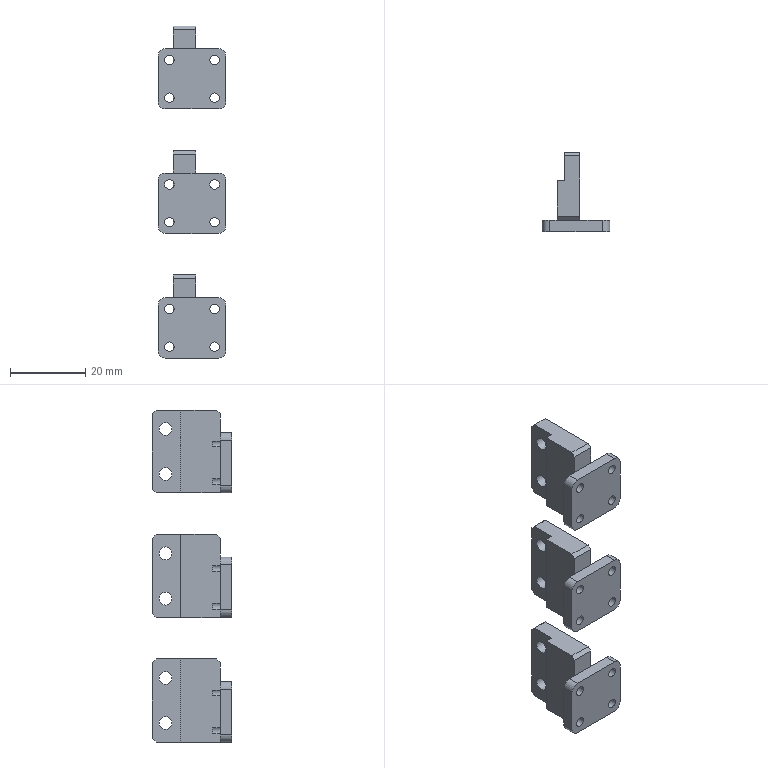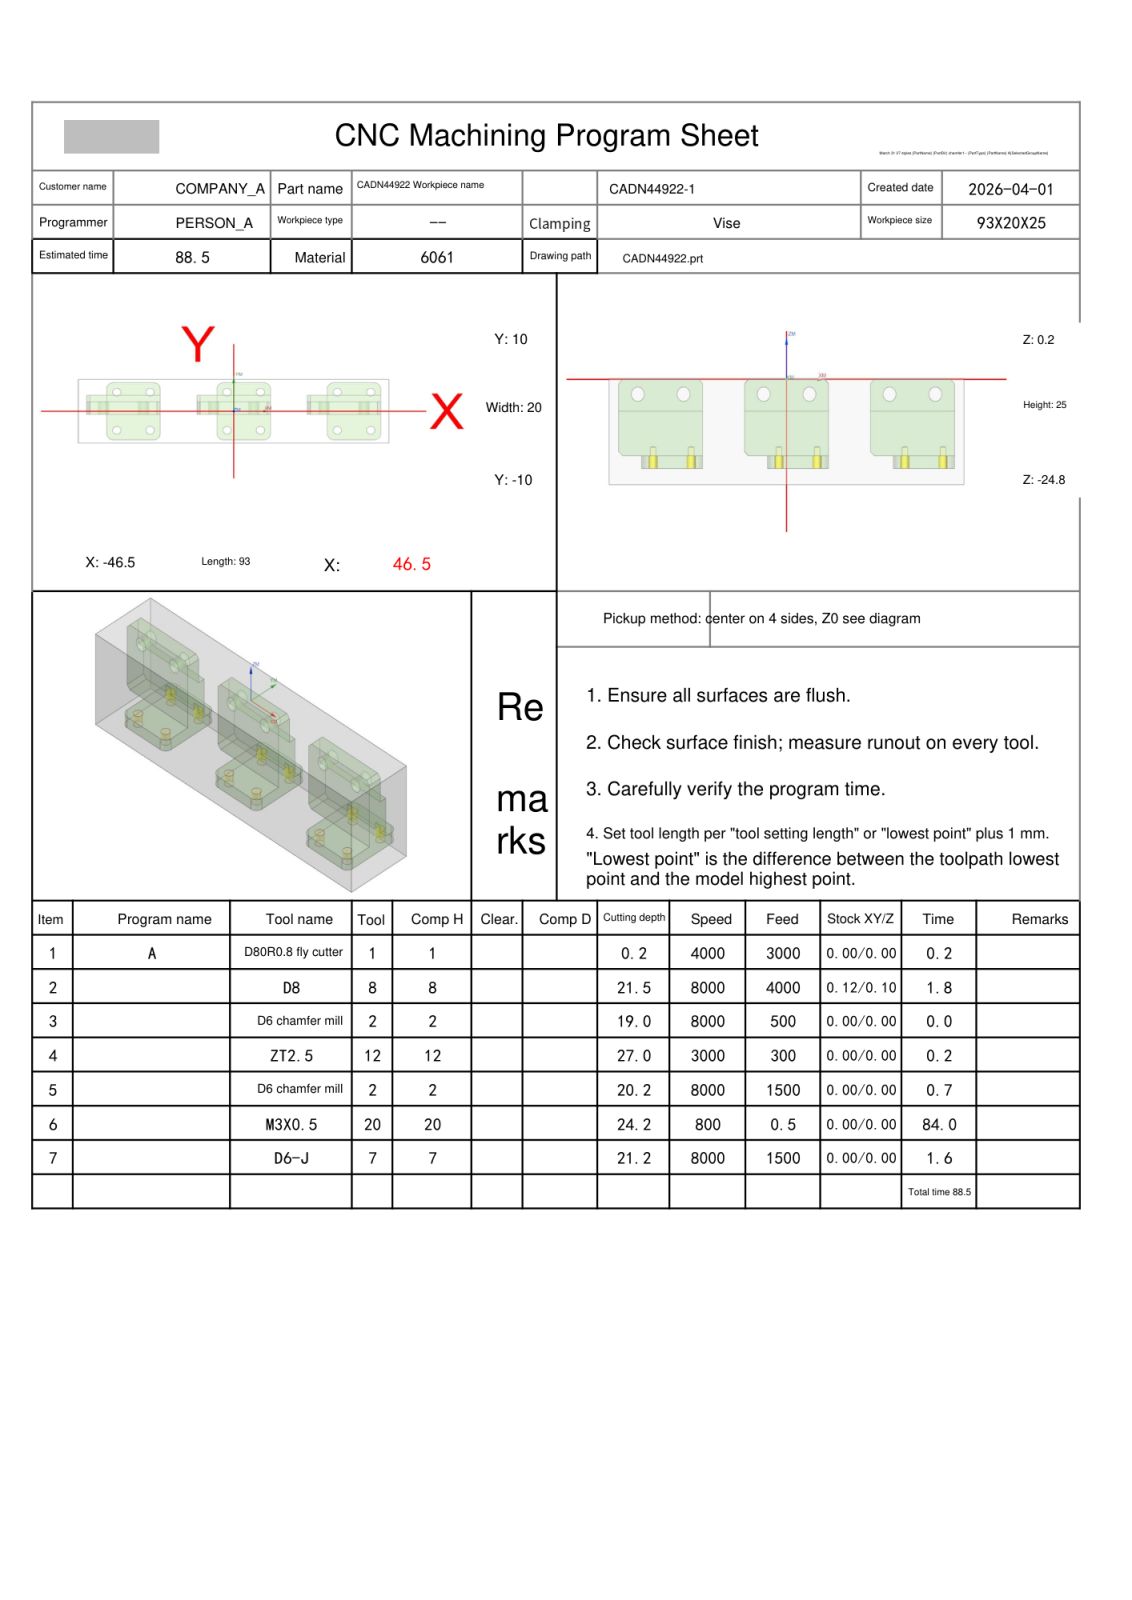NC program | NX | posted by the shop | part box 18 x 21 x 88 mm
Lines 42 to 965 of 4142:
N2 T08 M06
(D8  D=8. R=0. H=08 ce=0.12 di=0.10)
G00 G90 G54 X-55.984 Y.893 M03 S8000
G43 H08 Z20.
M08
Z-8.65
G01 X-55.886 Y.913 Z-9.275 F4000.
X-55.788 Y.933 Z-9.522
X-55.691 Y.953 Z-9.704
X-55.593 Y.973 Z-9.85
X-55.495 Y.993 Z-9.973
X-55.397 Y1.013 Z-10.078
X-55.299 Y1.033 Z-10.17
X-55.201 Y1.053 Z-10.25
X-55.103 Y1.073 Z-10.32
X-55.005 Y1.093 Z-10.382
X-54.907 Y1.114 Z-10.436
X-54.809 Y1.134 Z-10.483
X-54.711 Y1.154 Z-10.524
X-54.613 Y1.174 Z-10.558
X-54.515 Y1.194 Z-10.586
X-54.417 Y1.214 Z-10.61
X-54.319 Y1.234 Z-10.627
X-54.221 Y1.254 Z-10.64
X-54.123 Y1.274 Z-10.647
X-54.025 Y1.294 Z-10.65
G03 X-52.164 Y1.71 I-1.89 J12.828
X-51.742 Y2.726 I-1.554 J1.24
X-51.289 Y7.837 I-28.606 J5.111
X-51.291 Y8.113 I-29.059 J0.0
G01 Y8.202
G02 X-47.426 Y13.635 I5.75 J0.0
X-42.098 Y14.609 I5.697 J-16.103
X-32.642 Y14.767 I9.456 J-283.132
X-29.54 Y14.75 I0.0 J-283.29
G01 X44.939 Y14.729
G02 X50.005 Y11.176 I-.129 J-5.57
X51.093 Y5.793 I-14.693 J-5.771
X51.267 Y-3.345 I-239.376 J-9.138
X51.206 Y-8.763 I-239.55 J0.0
X47.747 Y-13.477 I-5.525 J.429
X42.45 Y-14.583 I-5.745 J14.271
X32.82 Y-14.772 I-9.629 J244.878
X29.493 Y-14.75 I0.0 J245.068
G01 X-44.987 Y-14.727
G02 X-50.03 Y-11.129 I.183 J5.591
X-51.097 Y-5.741 I15.012 J5.771
X-51.228 Y-2.403 I42.34 J3.339
X-51.135 Y.413 I42.471 J0.0
G03 X-50.486 Y7.409 I-193.07 J21.425
G02 X-46.65 Y12.332 I6.527 J-1.129
X-40.927 Y13.707 I6.529 J-14.588
X-32.915 Y13.956 I8.013 J-128.587
X-31.333 Y13.946 I0.0 J-128.836
G01 X43.227 Y13.93
G02 X48.701 Y10.316 I-.3 J-6.408
X50.166 Y4.775 I-13.357 J-6.497
X50.458 Y-3.345 I-112.899 J-8.12
X50.392 Y-7.216 I-113.19 J0.0
X46.802 Y-12.21 I-6.393 J.809
X41.187 Y-13.675 I-6.52 J13.493
X32.742 Y-13.964 I-8.445 J123.39
X30.714 Y-13.947 I0.0 J123.679
G01 X-43.285 Y-13.927
G02 X-48.694 Y-10.332 I.352 J6.396
X-50.172 Y-4.719 I13.363 J6.519
X-50.312 Y-1.795 I30.33 J2.925
X-50.173 Y1.111 I30.47 J0.0
X-49.729 Y6.084 I64.93 J-3.295
X-45.409 Y11.411 I7.394 J-1.582
X-39.138 Y12.893 I7.16 J-16.28
X-30.529 Y13.158 I8.609 J-140.056
X-28.744 Y13.146 I0.0 J-140.32
G01 X41.656 Y13.124
G02 X47.801 Y8.989 I-.403 J-7.234
X49.394 Y2.588 I-15.303 J-7.205
X49.628 Y-2.9 I-64.165 J-5.488
X49.569 Y-5.644 I-64.399 J0.0
X45.403 Y-11.344 I-7.201 J.891
X39.388 Y-12.861 I-7.037 J15.229
X30.46 Y-13.164 I-8.928 J131.417
X28.355 Y-13.147 I0.0 J131.72
G01 X-41.485 Y-13.133
G02 X-47.836 Y-8.926 I.241 J7.261
X-49.36 Y-2.003 I14.96 J6.923
X-49.358 Y-1.708 I16.484 J0.0
X-49.369 Y-.773 I38.904 J.935
X-48.975 Y4.753 I38.915 J0.0
X-44.084 Y10.609 I8.073 J-1.773
X-37.714 Y12.072 I7.44 J-17.796
X-28.909 Y12.355 I8.805 J-136.712
X-27.241 Y12.345 I0.0 J-136.995
G01 X40.039 Y12.323
G02 X46.809 Y8.02 I-.241 J-7.856
X48.159 Y5.123 I-3.267 J-3.285
X48.764 Y-2.392 I-46.345 J-7.515
X48.732 Y-4.123 I-46.951 J0.0
X44.329 Y-10.395 I-7.739 J.752
X38.016 Y-12.03 I-7.455 J15.78
X28.725 Y-12.364 I-9.291 J129.17
X26.585 Y-12.346 I0.0 J129.504
G01 X-39.975 Y-12.327
G02 X-47.003 Y-7.632 I.205 J7.916
X-48.407 Y-1.05 I14.735 J6.582
G01 X-48.406 Y-.95
G02 X-48.44 Y.203 I20.011 J1.154
X-48.12 Y3.769 I20.044 J0.0
X-48.135 Y4.318 I9.892 J.549
X-47.98 Y6.066 I9.907 J0.0
X-45.712 Y8.765 I4.256 J-1.274
X-37.316 Y11.193 I9.893 J-18.479
X-27.715 Y11.559 I9.602 J-125.917
X-25.806 Y11.544 I0.0 J-126.282
G01 X38.514 Y11.524
G02 X44.382 Y9.115 I-.093 J-8.581
G03 X45.066 Y8.98 I.887 J2.675
G02 X47.568 Y7.06 I-1.27 J-4.245
X48.12 Y4.998 I-4.216 J-2.233
X48.142 Y2.533 I-138.337 J-2.466
X48.074 Y-1.804 I-138.359 J0.0
X45.854 Y-7.572 I-8.758 J.06
X40.148 Y-10.643 I-7.988 J8.005
X32.366 Y-11.467 I-7.902 J37.493
X21.714 Y-11.551 I-10.652 J671.44
X19.887 Y-11.549 I0.0 J671.524
G01 X-38.513 Y-11.524
G02 X-46.253 Y-6.215 I.083 J8.418
X-47.08 Y-3.696 I21.506 J8.456
X-47.98 Y-2.066 I3.296 J2.883
G01 X-48.12 Y-1.
Y3.8
Y-1.
G03 X-46.913 Y-3.913 I4.433 J.13
X-44.908 Y-7.134 I34.469 J19.229
X-38.844 Y-10.524 I7.102 J5.587
X-32.41 Y-10.909 I6.434 J53.534
X-31.34 Y-10.898 I0.0 J53.919
G01 X29.14 Y-10.881
G03 X29.847 Y-10.885 I.706 J59.781
X38.153 Y-10.305 I0.0 J59.785
X43.773 Y-8.117 I-1.717 J12.722
X46.578 Y-4.211 I-4.972 J6.53
G01 X47.312 Y-3.451
X47.903 Y-2.319
X48.119 Y-1.062
X47.903 Y-2.319
X47.312 Y-3.451
G02 X44.255 Y-6.458 I-57.135 J55.023
X37.426 Y-9.418 I-8.966 J11.325
X28.955 Y-10.068 I-8.47 J54.924
X28.579 Y-10.066 I0.0 J55.573
G01 X18.099 Y-10.108
X-32.54 Y-10.08
G02 X-33.092 Y-10.085 I-.552 J31.482
X-38.749 Y-9.573 I0.0 J31.487
X-44.431 Y-5.798 I2.277 J9.59
G03 X-45.15 Y-4.945 I-6.698 J-4.918
G02 X-46.913 Y-3.913 I1.335 J4.305
G03 X-45.066 Y-4.98 I3.249 J3.495
G02 X-42.623 Y-6.82 I-24.322 J-34.837
G03 X-36.214 Y-9.123 I7.609 J11.103
X-28.807 Y-9.472 I7.407 J78.36
X-27.506 Y-9.461 I0.0 J78.709
G01 X27.214 Y-9.44
G03 X27.88 Y-9.443 I.666 J63.325
X36.467 Y-8.858 I0.0 J63.329
X44.555 Y-5.08 I-2.017 J14.86
G02 X45.262 Y-4.922 I.938 J-2.542
G01 X46.402 Y-4.347
X45.262 Y-4.922
G03 X42.996 Y-5.674 I.757 J-6.073
G02 X32.513 Y-8.399 I-11.731 J23.597
X22.846 Y-8.674 I-9.667 J169.882
X20.999 Y-8.664 I0.0 J170.156
G01 X-29.401 Y-8.642
G02 X-30.087 Y-8.648 I-.686 J42.
X-36.969 Y-8.08 I0.0 J42.005
X-42.722 Y-5.522 I3.391 J15.371
G03 X-43.802 Y-5.107 I-1.08 J-1.199
X-44.002 Y-5.12 I0.0 J-1.614
G01 X-45.066 Y-4.98
G03 X-43.144 Y-5.158 I3.33 J25.387
G02 X-39.892 Y-6.427 I-12.7 J-37.355
G03 X-32.05 Y-7.878 I8.484 J23.937
X-22.415 Y-8.041 I9.636 J284.651
X-19.573 Y-8.027 I0.0 J284.814
G01 X25.387 Y-7.999
G03 X26.124 Y-8.003 I.736 J68.243
X35.438 Y-7.365 I0.0 J68.247
X42.537 Y-5.145 I-5.252 J29.256
G01 X43.998 Y-5.12
X44.63 Y-5.021
G02 X42.923 Y-5.144 I-1.707 J11.757
X42.164 Y-5.12 I0.0 J11.881
G03 X38.031 Y-5.98 I4.598 J-32.461
G02 X27.071 Y-7.148 I-11.178 J52.874
X16.493 Y-7.23 I-10.578 J683.914
X14.352 Y-7.227 I0.0 J683.995
G01 X-27.168 Y-7.202
G02 X-27.827 Y-7.206 I-.659 J52.348
X-35.698 Y-6.611 I0.0 J52.353
X-40.837 Y-5.12 I6.892 J33.353
G01 X-43.397
G02 X-42.167 Y-5.095 I1.23 J-30.67
X-39.696 Y-5.195 I0.0 J-30.695
G03 X-33.218 Y-6.246 I15.885 J77.366
X-24.166 Y-6.591 I9.052 J118.887
X-22.747 Y-6.582 I0.0 J119.231
G01 X23.573 Y-6.561
G03 X24.392 Y-6.565 I.819 J79.441
X35.219 Y-5.824 I0.0 J79.446
G01 X38.762 Y-5.12
X42.202
G03 X39.693 Y-5.096 I-2.51 J-132.267
X35.211 Y-5.172 I0.0 J-132.291
G02 X20.435 Y-5.789 I-14.776 J176.515
X18.622 Y-5.78 I0.0 J177.132
G01 X-25.138 Y-5.762
G02 X-25.772 Y-5.765 I-.634 J70.43
X-35.285 Y-5.12 I0.0 J70.433
G01 X-40.485
X21.244 Y-5.126
X36.158 Y-5.12
X21.998
G02 X19.916 Y-4.721 I1.575 J13.876
G03 X14.411 Y-4.368 I-5.504 J-42.74
X13.376 Y-4.381 I0.0 J-43.093
G02 X10.998 Y-5.12 I-2.59 J4.136
G01 X-11.002
G02 X-13.232 Y-4.7 I2.272 J18.19
G03 X-18.518 Y-4.371 I-5.286 J-42.35
X-19.664 Y-4.386 I0.0 J-42.678
G01 X-20.755 Y-4.928
X-22.002 Y-5.12
X-20.755 Y-4.928
G02 X-18.492 Y-4.072 I3.398 J-5.57
X-16.287 Y-3.922 I2.206 J-16.071
X-13.635 Y-4.14 I0.0 J-16.222
G03 X-12.099 Y-4.966 I2.816 J3.395
G02 X-13.719 Y-4.062 I1.239 J4.125
G03 X-16.7 Y-3.375 I-2.981 J-6.124
X-17.019 Y-3.383 I0.0 J-6.811
G01 X-17.077
G03 X-18.794 Y-3.593 I0.0 J-7.099
G01 X-19.627 Y-4.368
G02 X-18.605 Y-3.451 I4.484 J-3.973
X-16.408 Y-3.018 I2.197 J-5.35
X-14.336 Y-3.401 I0.0 J-5.784
G03 X-13.659 Y-4.108 I3.262 J2.447
G02 X-14.354 Y-3.346 I1.716 J2.262
G03 X-16.7 Y-2.595 I-2.346 J-3.29
X-17.412 Y-2.658 I0.0 J-4.041
X-18.427 Y-2.991 I.135 J-2.126
G02 X-18.836 Y-3.605 I-3.058 J1.594
G03 X-18.402 Y-2.93 I-2.393 J2.014
G02 X-16.487 Y-2.316 I1.915 J-2.683
X-15.623 Y-2.431 I0.0 J-3.297
X-14.631 Y-2.909 I-.133 J-1.546
G03 X-14.276 Y-3.441 I2.812 J1.492
G02 X-14.775 Y-2.682 I7.022 J5.161
G03 X-16.661 Y-1.996 I-1.886 J-2.252
X-18.072 Y-2.357 I0.0 J-2.937
G01 X-18.457 Y-3.008
G02 X-17.93 Y-2.196 I2.254 J-.885
X-16.492 Y-1.778 I1.438 J-2.268
X-14.921 Y-2.286 I0.0 J-2.686
G01 X-14.664 Y-2.828
G03 X-16.378 Y-1.51 I-1.722 J-.466
X-16.7 Y-1.483 I-.322 J-1.937
X-18.001 Y-1.977 I0.0 J-1.963
G01 X-18.12 Y-2.387
G02 X-17.266 Y-1.422 I1.058 J-.076
X-16.516 Y-1.293 I.749 J-2.107
X-15.08 Y-1.815 I0.0 J-2.237
G01 X-14.857 Y-2.362
G03 X-15.183 Y-1.615 I-2.709 J-.739
X-16.582 Y-1.03 I-1.399 J-1.379
X-17.93 Y-1.566 I0.0 J-1.964
G01 X-18.075 Y-2.152
Y-2.14
G02 X-17.004 Y-.926 I1.223 J0.0
X-16.505 Y-.858 I.499 J-1.795
X-15.08 Y-1.521 I0.0 J-1.863
G01 X-14.995 Y-1.948
G03 X-16.063 Y-.706 I-1.264 J-.007
X-16.593 Y-.628 I-.529 J-1.759
X-17.827 Y-1.105 I0.0 J-1.837
X-17.995 Y-1.734 I2.468 J-.996
G02 X-17.747 Y-.951 I1.47 J-.035
X-16.513 Y-.463 I1.233 J-1.315
X-15.144 Y-1.094 I0.0 J-1.803
G01 X-15.039 Y-1.617
X-15.038 Y-1.573
G03 X-16.19 Y-.289 I-1.291 J0.0
X-16.629 Y-.226 I-.439 J-1.493
X-17.839 Y-.805 I0.0 J-1.556
G01 X-17.898 Y-1.231
X-17.903 Y-1.132
G02 X-17.167 Y-.201 I.957 J0.0
X-16.515 Y-.069 I.653 J-1.542
X-15.156 Y-.764 I0.0 J-1.674
G01 X-15.099 Y-1.159
X-15.097 Y-1.087
G03 X-15.991 Y.035 I-1.15 J0.0
X-16.576 Y.143 I-.585 J-1.532
X-17.826 Y-.436 I0.0 J-1.64
X-17.885 Y-.871 I1.594 J-.435
G01 X-17.883 Y-.94
X-17.899 Y-.768
G02 X-17.196 Y.159 I.962 J0.0
X-16.52 Y.303 I.676 J-1.505
X-15.151 Y-.426 I0.0 J-1.65
G01 X-15.12 Y-.868
X-15.108 Y-.702
G03 X-16.001 Y.407 I-1.136 J0.0
X-16.581 Y.518 I-.58 J-1.467
X-17.843 Y-.114 I0.0 J-1.577
X-17.883 Y-.657 I3.821 J-.553
G02 X-17.902 Y-.456 I1.04 J.201
X-17. Y.592 I1.06 J0.0
X-16.507 Y.669 I.493 J-1.545
X-15.151 Y-.063 I0.0 J-1.622
G01 X-15.12 Y-.505
X-15.107 Y-.336
G03 X-15.988 Y.772 I-1.138 J0.0
X-16.574 Y.884 I-.586 J-1.483
X-17.837 Y.261 I0.0 J-1.594
X-17.883 Y-.251 I2.83 J-.512
G01 Y-.307
G02 X-17.904 Y-.096 I1.046 J.212
X-17.007 Y.957 I1.067 J0.0
X-16.507 Y1.036 I.5 J-1.545
X-15.154 Y.309 I0.0 J-1.624
G01 X-15.12 Y-.139
X-15.107 Y.031
G03 X-15.978 Y1.136 I-1.137 J0.0
X-16.581 Y1.258 I-.603 J-1.431
X-17.849 Y.601 I0.0 J-1.553
G01 X-17.883 Y.155
X-17.897 Y.32
G02 X-17.188 Y1.264 I.983 J0.0
X-16.52 Y1.406 I.668 J-1.498
X-15.151 Y.67 I0.0 J-1.64
G01 X-15.12 Y.228
X-15.107 Y.398
G03 X-15.978 Y1.504 I-1.137 J0.0
X-16.573 Y1.618 I-.594 J-1.491
X-17.832 Y1.007 I0.0 J-1.605
X-17.885 Y.533 I2.129 J-.475
G01 X-17.882 Y.433
G02 X-17.903 Y.643 I1.045 J.211
X-17.031 Y1.692 I1.066 J0.0
X-16.516 Y1.775 I.515 J-1.554
X-15.154 Y1.046 I0.0 J-1.637
G01 X-15.12 Y.597
X-15.108 Y.763
G03 X-16.006 Y1.882 I-1.147 J0.0
X-16.574 Y1.987 I-.568 J-1.491
X-17.836 Y1.369 I0.0 J-1.596
X-17.882 Y.878 I2.964 J-.528
G01 X-17.899 Y1.059
G02 X-17.211 Y1.991 I.976 J0.0
X-16.509 Y2.154 I.702 J-1.427
X-15.14 Y1.373 I0.0 J-1.59
G01 X-15.12 Y.957
X-15.106 Y1.132
G03 X-15.98 Y2.242 I-1.142 J0.0
X-16.571 Y2.354 I-.591 J-1.496
X-17.833 Y1.745 I0.0 J-1.609
X-17.882 Y1.264 I2.318 J-.481
G01 Y1.251
X-17.899 Y1.432
G02 X-17.212 Y2.36 I.971 J0.0
X-16.524 Y2.509 I.689 J-1.517
X-15.162 Y1.803 I0.0 J-1.666
X-15.12 Y1.333 I-3.591 J-.559
G01 X-15.107 Y1.502
G03 X-15.98 Y2.611 I-1.141 J0.0
X-16.571 Y2.723 I-.59 J-1.494
X-17.833 Y2.11 I0.0 J-1.606
X-17.882 Y1.619 I2.454 J-.491
G01 Y1.617
X-17.894 Y1.777
G02 X-17.105 Y2.772 I1.022 J0.0
X-16.512 Y2.885 I.593 J-1.5
X-15.146 Y2.129 I0.0 J-1.613
G01 X-15.12 Y1.699
X-15.107 Y1.871
G03 X-15.979 Y2.979 I-1.14 J0.0
X-16.582 Y3.101 I-.603 J-1.425
X-17.848 Y2.443 I0.0 J-1.547
G01 X-17.882 Y1.997
X-17.896 Y2.162
G02 X-17.186 Y3.107 I.984 J0.0
X-16.52 Y3.248 I.666 J-1.499
X-15.151 Y2.511 I0.0 J-1.64
G01 X-15.12 Y2.07
X-15.107 Y2.24
G03 X-15.979 Y3.347 I-1.139 J0.0
X-16.571 Y3.459 I-.592 J-1.495
X-17.836 Y2.843 I0.0 J-1.608
X-17.882 Y2.324 I2.95 J-.519
G01 X-17.881 Y2.275
G02 X-17.902 Y2.484 I1.044 J.21
X-17.003 Y3.536 I1.065 J0.0
X-16.508 Y3.614 I.495 J-1.549
X-15.154 Y2.887 I0.0 J-1.626
G01 X-15.12 Y2.439
X-15.107 Y2.608
G03 X-15.979 Y3.715 I-1.139 J0.0
X-16.569 Y3.827 I-.59 J-1.49
X-17.835 Y3.207 I0.0 J-1.603
X-17.881 Y2.718 I3.153 J-.542
G01 X-17.894 Y2.878
G02 X-17.096 Y3.891 I1.042 J0.0
X-16.522 Y3.997 I.575 J-1.498
X-15.142 Y3.212 I0.0 J-1.604
G01 X-15.12 Y2.79
X-15.109 Y2.952
G03 X-16.129 Y4.155 I-1.219 J0.0
X-16.576 Y4.22 I-.447 J-1.49
X-17.845 Y3.564 I0.0 J-1.556
G01 X-17.881 Y3.111
X-17.891 Y3.257
G02 X-17.003 Y4.315 I1.075 J0.0
X-16.518 Y4.391 I.485 J-1.513
X-15.141 Y3.596 I0.0 J-1.589
G01 X-15.12 Y3.176
X-15.11 Y3.331
G03 X-16.267 Y4.586 I-1.259 J0.0
X-16.594 Y4.622 I-.327 J-1.462
X-17.852 Y3.937 I0.0 J-1.498
G01 X-17.881 Y3.422
G02 X-17.899 Y3.622 I1.109 J.2
X-16.936 Y4.737 I1.126 J0.0
X-16.517 Y4.793 I.419 J-1.531
X-15.143 Y4. I0.0 J-1.587
G01 X-15.12 Y3.497
G03 X-15.103 Y3.706 I-1.287 J.209
X-16.407 Y5.009 I-1.304 J0.0
G01 X-16.409
G03 X-16.634 Y5.027 I-.225 J-1.382
X-17.864 Y4.297 I0.0 J-1.4
G01 X-17.881 Y3.743
G02 X-17.905 Y3.987 I1.196 J.244
X-17.661 Y4.719 I1.221 J0.0
X-16.52 Y5.21 I1.142 J-1.082
X-15.137 Y4.386 I0.0 J-1.573
G01 X-15.12 Y3.912
G03 X-15.102 Y4.124 I-1.277 J.212
X-16.395 Y5.418 I-1.295 J0.0
X-16.627 Y5.437 I-.232 J-1.402
X-17.859 Y4.725 I0.0 J-1.421
G01 X-17.88 Y4.226
G02 X-17.789 Y5.659 I43.024 J-2.025
G03 X-20.287 Y9.349 I-4.719 J-.503
X-25.102 Y10.687 I-5.356 J-9.946
X-30.065 Y10.87 I-4.962 J-67.001
X-38.594 Y10.327 I0.0 J-67.184
X-43.183 Y9.12 I3.439 J-22.406
X-43.671 Y9.143 I-.488 J-5.23
X-46.06 Y8.568 I0.0 J-5.253
G02 X-43.671 Y9.143 I2.389 J-4.678
X-43.183 Y9.12 I0.0 J-5.252
G03 X-39.086 Y9.472 I-.17 J26.04
G02 X-30.028 Y10.034 I9.058 J-72.709
X-26.391 Y9.943 I0.0 J-73.271
X-22.46 Y9.12 I-.744 J-13.344
X-22.173 Y9.129 I.287 J-4.516
X-19.087 Y7.913 I0.0 J-4.525
X-17.876 Y4.866 I-3.229 J-3.047
G01 X-17.88 Y4.678
X-17.877 Y4.858
G03 X-19.087 Y7.913 I-4.462 J0.0
X-22.174 Y9.129 I-3.087 J-3.312
X-22.46 Y9.12 I0.0 J-4.527
G02 X-27.808 Y9.347 I5.551 J193.932
G03 X-29.304 Y9.359 I-1.496 J-90.788
X-35.89 Y9.12 I0.0 J-90.8
G01 X-42.37
X-23.25
G03 X-22.953 Y9.252 I-.008 J.419
G01 X-22.416 Y9.848
X-21.364 Y11.016 Z-10.55
X-20.921 Y11.509
X-20.87 Y11.556
X-20.813 Y11.593
X-20.75 Y11.62
X-16.09 Y13.174
X-15.623 Y13.325
X-15.153 Y13.467
X-14.681 Y13.6
X-14.206 Y13.725
X-13.934 Y13.789
X-13.66 Y13.844
X-13.385 Y13.889
X-13.108 Y13.925
X-12.83 Y13.951
X-12.551 Y13.968
X-12.271 Y13.975
X37.312 Y14.411
X37.689 Y14.409
X38.065 Y14.395
X38.441 Y14.371
X38.816 Y14.336
X39.189 Y14.29
X39.562 Y14.233
X39.932 Y14.165
X40.3 Y14.087
X40.666 Y13.998
X41.029 Y13.898
X41.389 Y13.787
X41.746 Y13.666
X42.099 Y13.535
X44.544 Y12.585
X44.602 Y12.557
X44.655 Y12.52
X44.701 Y12.475
X44.739 Y12.423
X44.768 Y12.365
X44.788 Y12.304
X44.798 Y12.24
X44.886 Y10.999
X44.996 Y9.431 Z-10.65
G02 X44.595 Y9.045 I-.4 J.015
G01 X44.544 Y9.048
G02 X42.149 Y9.958 I10.936 J32.404
G03 X36.185 Y10.837 I-5.965 J-19.782
G01 X36.076
G03 X26.709 Y10.908 I-9.367 J-615.807
G01 X26.157
X-10.64 Y10.888
G03 X-13.243 Y8.707 I.895 J-3.712
G02 X-13.913 Y7.913 I-1.332 J.445
G03 X-15.12 Y5.002 I3.22 J-3.04
G01 Y4.362
G02 X-15.134 Y4.738 I5.032 J.377
X-14.568 Y7.06 I5.046 J0.0
X-11.746 Y9.152 I4.124 J-2.613
X-5.91 Y10.013 I5.892 J-19.741
X.442 Y10.12 I6.352 J-188.533
X2.569 Y10.108 I0.0 J-188.64
G01 X34.488 Y10.084
G02 X34.898 Y10.087 I.409 J-23.458
X41.566 Y9.12 I0.0 J-23.462
X42.575 Y9.144 I1.008 J-20.805
X44.478 Y9.057 I0.0 J-20.829
G03 X42.575 Y9.144 I-1.903 J-20.742
X41.566 Y9.12 I0.0 J-20.829
G02 X36.368 Y9.358 I1.498 J89.466
G03 X25.671 Y9.474 I-10.697 J-492.923
X23.089 Y9.467 I0.0 J-493.039
G01 X-3.07 Y9.443
G03 X-8.415 Y9.12 I.403 J-51.051
G01 X-10.998
G03 X-13.06 Y8.568 I.172 J-4.77
G02 X-10.998 Y9.12 I2.233 J-4.216
G01 X11.002
G03 X17.523 Y8.683 I6.521 J48.497
X18.201 Y8.688 I0.0 J48.934
G01 X20.245 Y8.695
G02 X22.002 Y9.12 I1.87 J-3.883
G01 X40.562
G03 X40.962 Y9.52 I0.0 J.4
X40.776 Y9.858 I-.4 J0.0
G01 X40.183 Y10.233
X38.855 Y11.075 Z-10.55
X38.586 Y11.246
X38.537 Y11.272
X38.484 Y11.292
X38.43 Y11.304
X38.374 Y11.308
X21.793 Y11.374
X21.726 Y11.369
X21.662 Y11.353
X21.601 Y11.326
X21.545 Y11.29
X21.496 Y11.245
X21.455 Y11.192
X21.424 Y11.133
X21.385 Y11.044
X20.761 Y9.602 Z-10.65
X20.431 Y8.851
G02 X19.338 Y8.423 I-1.244 J1.567
X15.814 Y8.167 I-3.524 J24.144
X13.486 Y8.278 I0.0 J24.4
G03 X12.066 Y8.98 I-3.028 J-4.34
G02 X13.655 Y8.153 I-1.738 J-5.282
G03 X16.937 Y7.576 I3.282 J9.052
X17.91 Y7.626 I0.0 J9.629
G01 X18.026 Y7.623
G03 X19.002 Y7.828 I0.0 J2.426
G02 X20.088 Y8.629 I3.848 J-4.077
G03 X18.946 Y7.755 I1.868 J-3.621
G02 X16.47 Y7.195 I-2.476 J5.203
X15.758 Y7.239 I0.0 J5.762
X14.179 Y7.586 I.001 J3.771
G03 X13.406 Y8.303 I-2.221 J-1.622
G02 X14.24 Y7.498 I-1.443 J-2.332
G03 X16.675 Y6.761 I2.435 J3.653
X17.295 Y6.805 I0.0 J4.39
X18.495 Y7.142 I-.02 J2.375
G01 X19.079 Y7.903
G02 X18.244 Y6.919 I-3.856 J2.424
X16.461 Y6.468 I-1.783 J3.296
X14.664 Y6.927 I0.0 J3.748
G01 X14.178 Y7.568
G03 X14.907 Y6.656 I4.149 J2.569
X16.63 Y6.124 I1.722 J2.52
X18.186 Y6.55 I0.0 J3.053
G01 X18.481 Y7.123
G02 X18.056 Y6.384 I-2.15 J.742
X16.499 Y5.887 I-1.557 J2.189
X14.828 Y6.47 I0.0 J2.686
G01 X14.607 Y6.966
G03 X16.134 Y5.662 I1.682 J.423
X16.655 Y5.602 I.52 J2.218
X17.976 Y6.024 I0.0 J2.278
G01 X18.285 Y6.705
G02 X17.858 Y5.861 I-2.25 J.609
X16.487 Y5.407 I-1.371 J1.843
X15.077 Y5.89 I0.0 J2.297
G01 X14.796 Y6.51
G03 X15.24 Y5.643 I2.099 J.527
X16.581 Y5.145 I1.341 J1.558
X17.9 Y5.625 I0.0 J2.055
X18.02 Y6.066 I-1.34 J.602
G01 X18.021 Y6.045
G02 X17.37 Y5.156 I-.932 J0.0
X16.518 Y4.96 I-.851 J1.746
X15.07 Y5.607 I0.0 J1.943
G01 X14.98 Y6.066
X14.979 Y6.045
G03 X15.968 Y4.835 I1.235 J0.0
X16.591 Y4.724 I.623 J1.684
X17.873 Y5.263 I0.0 J1.795
X17.996 Y5.879 I-2.982 J.914
G01 X17.997 Y5.818
G02 X17.784 Y5.084 I-1.37 J0.0
X16.513 Y4.555 I-1.271 J1.263
X15.113 Y5.229 I0.0 J1.792
G01 X15.035 Y5.646
G03 X16.177 Y4.389 I1.271 J.008
X16.604 Y4.333 I.427 J1.614
X17.825 Y4.864 I0.0 J1.67
X17.943 Y5.478 I-5.741 J1.419
G01 X17.945 Y5.4
G02 X16.794 Y4.202 I-1.199 J0.0
X16.485 Y4.173 I-.309 J1.628
X15.164 Y4.83 I0.0 J1.657
G01 X15.078 Y5.316
X15.076 Y5.244
G03 X16.16 Y4.014 I1.239 J0.0
X16.593 Y3.954 I.432 J1.526
X17.832 Y4.55 I0.0 J1.586
X17.88 Y5.002 I-2.768 J.526
G01 X17.892 Y4.855
G02 X17.191 Y3.938 I-.95 J0.0
X16.514 Y3.791 I-.677 J1.494
X15.149 Y4.522 I0.0 J1.64
G01 X15.12 Y4.959
X15.107 Y4.791
G03 X15.991 Y3.69 I1.128 J0.0
X16.585 Y3.573 I.594 J1.446
X17.844 Y4.209 I0.0 J1.563
G01 X17.88 Y4.664
X17.894 Y4.501
G02 X17.165 Y3.557 I-.975 J0.0
X16.509 Y3.417 I-.655 J1.46
X15.143 Y4.184 I0.0 J1.601
G01 X15.12 Y4.606
X15.106 Y4.431
G03 X15.971 Y3.329 I1.134 J0.0
X16.568 Y3.217 I.597 J1.527
X17.82 Y3.798 I0.0 J1.64
X17.887 Y4.246 I-1.466 J.448
G01 X17.88 Y4.388
G02 X17.899 Y4.186 I-1.063 J-.202
X17.017 Y3.123 I-1.082 J0.0
X16.52 Y3.045 I-.498 J1.547
X15.148 Y3.798 I0.0 J1.626
G01 X15.12 Y4.232
X15.11 Y4.075
G03 X16.153 Y2.876 I1.21 J0.0
X16.586 Y2.814 I.433 J1.46
X17.85 Y3.487 I0.0 J1.522
G01 X17.88 Y4.006
G02 X17.899 Y3.805 I-1.082 J-.201
X16.986 Y2.72 I-1.101 J0.0
X16.514 Y2.649 I-.472 J1.531
X15.146 Y3.417 I0.0 J1.602
G01 X15.12 Y3.846
X15.111 Y3.694
G03 X16.269 Y2.451 I1.247 J0.0
X16.595 Y2.415 I.326 J1.444
X17.856 Y3.121 I0.0 J1.48
G01 X17.88 Y3.626
G02 X17.898 Y3.424 I-1.122 J-.202
X16.881 Y2.29 I-1.14 J0.0
X16.47 Y2.232 I-.41 J1.417
X15.128 Y3.094 I0.0 J1.475
G01 X15.12 Y3.451
X15.111 Y3.298
G03 X16.305 Y2.04 I1.26 J0.0
X16.619 Y2.005 I.314 J1.374
X17.866 Y2.757 I0.0 J1.409
G01 X17.88 Y3.22
X17.896 Y3.028
G02 X16.783 Y1.864 I-1.166 J0.0
X16.473 Y1.831 I-.311 J1.467
X15.135 Y2.654 I0.0 J1.5
G01 X15.12 Y3.119
G03 X15.102 Y2.908 I1.269 J-.211
X16.389 Y1.621 I1.286 J0.0
G01 X16.399
G03 X16.602 Y1.607 I.203 J1.475
X17.849 Y2.281 I0.0 J1.489
G01 X17.88 Y2.884
G02 X17.903 Y2.639 I-1.286 J-.245
X17.716 Y1.964 I-1.31 J0.0
X16.516 Y1.425 I-1.2 J1.066
X15.147 Y2.191 I0.0 J1.605
G01 X15.12 Y2.704
G02 X15.14 Y.854 I-83.805 J-1.85
X15.12 Y-1.002 I-83.825 J0.0
X13.913 Y-3.913 I-4.425 J.128
G01 X13.215 Y-4.449
G03 X14.568 Y-3.06 I-2.46 J3.749
X15.12 Y-1.002 I-4.214 J2.233
G01 Y2.24
G02 X15.525 Y2.683 I.445 J-.001
G01 X17.464 Y2.847
G02 X17.88 Y2.404 I-.029 J-.444
G03 X17.741 Y1.136 I28.161 J-3.731
X17.88 Y.152 I16.871 J1.881
X17.867 Y-.353 I9.625 J-.505
X18.02 Y-2.066 I9.638 J0.0
X19.94 Y-4.568 I4.244 J1.269
G01 X20.901 Y-4.966
G02 X18.432 Y-3.06 I1.257 J4.181
X17.88 Y-1. I4.217 J2.234
G01 X17.863 Y2.443
X16.449 Y7.654
X16.423 Y7.751 Z-10.647
X16.396 Y7.847 Z-10.64
X16.37 Y7.944 Z-10.627
X16.344 Y8.04 Z-10.61
X16.318 Y8.137 Z-10.586
X16.292 Y8.233 Z-10.558
X16.265 Y8.33 Z-10.524
X16.239 Y8.426 Z-10.483
X16.213 Y8.523 Z-10.436
X16.187 Y8.619 Z-10.382
X16.161 Y8.716 Z-10.32
X16.135 Y8.812 Z-10.25
X16.108 Y8.909 Z-10.17
X16.082 Y9.005 Z-10.078
X16.056 Y9.102 Z-9.973
X16.03 Y9.198 Z-9.85
X16.004 Y9.295 Z-9.704
X15.977 Y9.391 Z-9.522
X15.951 Y9.488 Z-9.275
X15.925 Y9.584 Z-8.65
G00 Z20.
X-16.834 Y9.711
Z-5.261
G01 X-16.822 Y9.612 Z-5.886
X-16.809 Y9.513 Z-6.133
X-16.796 Y9.414 Z-6.315
X-16.784 Y9.314 Z-6.461
X-16.771 Y9.215 Z-6.584
X-16.759 Y9.116 Z-6.69
X-16.746 Y9.017 Z-6.781
X-16.733 Y8.918 Z-6.861
X-16.721 Y8.818 Z-6.932
X-16.708 Y8.719 Z-6.993
X-16.695 Y8.62 Z-7.047
X-16.683 Y8.521 Z-7.094
X-16.67 Y8.422 Z-7.135
X-16.658 Y8.322 Z-7.169
X-16.645 Y8.223 Z-7.198
X-16.632 Y8.124 Z-7.221
X-16.62 Y8.025 Z-7.239
X-16.607 Y7.926 Z-7.251
X-16.594 Y7.826 Z-7.259
X-16.582 Y7.727 Z-7.261
X-16.045 Y3.509
G03 X-15.549 Y3.072 I.496 J.063
X-15.053 Y3.507 I0.0 J.5
G02 X-13.228 Y6.439 I3.916 J-.403
X-8.903 Y7.912 I5.273 J-8.396
X-2.72 Y8.273 I6.183 J-52.763
X-1.957 Y8.268 I0.0 J-53.124
X3.642 Y8.291 I5.599 J-664.749
X9.179 Y8.268 I0.0 J-664.772
X11.579 Y7.09 I-.579 J-4.212
X13.06 Y6.568 I-1.916 J-7.801
X14.98 Y4.066 I-2.324 J-3.771
G01 X15.063 Y3.432
G03 X14.568 Y5.06 I-4.174 J-.38
X12.066 Y6.98 I-3.771 J-2.324
X5.463 Y7.624 I-6.603 J-33.49
X4.902 Y7.62 I0.0 J-34.135
X1.416 Y7.658 I-3.485 J-158.512
X-6.614 Y7.455 I0.0 J-158.55
X-9.104 Y7.12 I3.443 J-35.036
X-9.89 Y7.141 I-.786 J-14.742
X-12.066 Y6.98 I0.0 J-14.763
G01 X-13.06 Y6.568
G02 X-10.998 Y7.12 I2.233 J-4.216
G01 X11.002
X11.715 Y7.026
X11.768 Y7.022
G03 X12.168 Y7.422 I0.0 J.4
X11.979 Y7.762 I-.4 J0.0
G01 X11.204 Y8.244
X9.869 Y9.073 Z-7.161
X9.74 Y9.154
X9.691 Y9.18
X9.638 Y9.199
X9.583 Y9.21
X9.527 Y9.214
X-11.681 Y9.119
X-11.742 Y9.114
X-11.802 Y9.1
X-11.859 Y9.076
X-11.911 Y9.045
X-11.958 Y9.005
X-12.095 Y8.784 Z-7.178
X-12.2 Y8.547 Z-7.194
X-12.642 Y7.593 Z-7.261
X-13.14 Y6.532
X-13.228 Y6.439
X-13.913 Y5.913
G02 X-14.159 Y5.83 I-.246 J.322
X-14.486 Y5.996 I0.0 J.405
G01 X-15.37 Y7.212
X-15.428 Y7.293 Z-7.259
X-15.487 Y7.373 Z-7.251
X-15.546 Y7.454 Z-7.239
X-15.605 Y7.535 Z-7.221
X-15.663 Y7.616 Z-7.198
X-15.722 Y7.697 Z-7.169
X-15.781 Y7.778 Z-7.135
X-15.84 Y7.859 Z-7.094
X-15.899 Y7.94 Z-7.047
X-15.957 Y8.021 Z-6.993
X-16.016 Y8.101 Z-6.932
X-16.075 Y8.182 Z-6.861
X-16.134 Y8.263 Z-6.781
X-16.193 Y8.344 Z-6.69
X-16.251 Y8.425 Z-6.584
X-16.31 Y8.506 Z-6.461
X-16.369 Y8.587 Z-6.315
X-16.428 Y8.668 Z-6.133
X-16.487 Y8.749 Z-5.886
X-16.545 Y8.829 Z-5.261
G00 Z20.
X-52.08 Y2.951
Z-5.261
G01 X-51.98 Y2.956 Z-5.886
X-51.88 Y2.96 Z-6.133
X-51.781 Y2.964 Z-6.315
X-51.681 Y2.969 Z-6.461
X-51.581 Y2.973 Z-6.584
X-51.481 Y2.978 Z-6.69
X-51.381 Y2.982 Z-6.781
X-51.281 Y2.987 Z-6.861
X-51.181 Y2.991 Z-6.932
X-51.081 Y2.995 Z-6.993
X-50.981 Y3. Z-7.047
X-50.881 Y3.004 Z-7.094
X-50.782 Y3.009 Z-7.135
X-50.682 Y3.013 Z-7.169
X-50.582 Y3.017 Z-7.198
X-50.482 Y3.022 Z-7.221
X-50.382 Y3.026 Z-7.239
X-50.282 Y3.031 Z-7.251
X-50.182 Y3.035 Z-7.259
X-50.082 Y3.039 Z-7.261
X-48.446 Y3.112
G03 X-48.058 Y3.448 I-.02 J.415
G01 X-47.885 Y4.372
X-47.286 Y5.485
G02 X-43.996 Y7.477 I4.8 J-4.216
X-38.022 Y8.223 I5.973 J-23.546
G01 X-37.898 Y8.222
G02 X-29.085 Y8.281 I8.813 J-659.832
X-23.817 Y8.26 I0.0 J-659.89
X-21.417 Y7.083 I-.568 J-4.193
X-19.94 Y6.568 I-1.574 J-6.886
X-18.02 Y4.066 I-2.324 J-3.771
G01 X-17.937 Y3.432
G03 X-18.432 Y5.06 I-4.174 J-.38
X-20.934 Y6.98 I-3.771 J-2.324
X-27.795 Y7.628 I-6.862 J-35.968
X-28.521 Y7.621 I0.0 J-36.617
X-31.901 Y7.659 I-3.38 J-149.14
X-39.717 Y7.455 I0.0 J-149.178
X-42.144 Y7.12 I3.484 J-34.254
X-42.916 Y7.144 I-.772 J-12.603
X-45.248 Y6.926 I0.0 J-12.626
G01 X-46.379 Y6.364
X-45.248 Y6.926
G02 X-42.916 Y7.144 I2.332 J-12.409
X-42.144 Y7.12 I0.0 J-12.626
G01 X-21.998
X-21.285 Y7.026
X-21.233 Y7.022
G03 X-20.842 Y7.314 I0.0 J.408
G01 X-20.388 Y8.85
X-20.359 Y8.946 Z-7.259
X-20.331 Y9.042 Z-7.251
X-20.303 Y9.138 Z-7.239
X-20.274 Y9.233 Z-7.221
X-20.246 Y9.329 Z-7.198
X-20.218 Y9.425 Z-7.169
X-20.189 Y9.521 Z-7.135
X-20.161 Y9.617 Z-7.094
X-20.133 Y9.713 Z-7.047
X-20.104 Y9.809 Z-6.993
X-20.076 Y9.905 Z-6.932
X-20.048 Y10.001 Z-6.861
X-20.019 Y10.097 Z-6.781